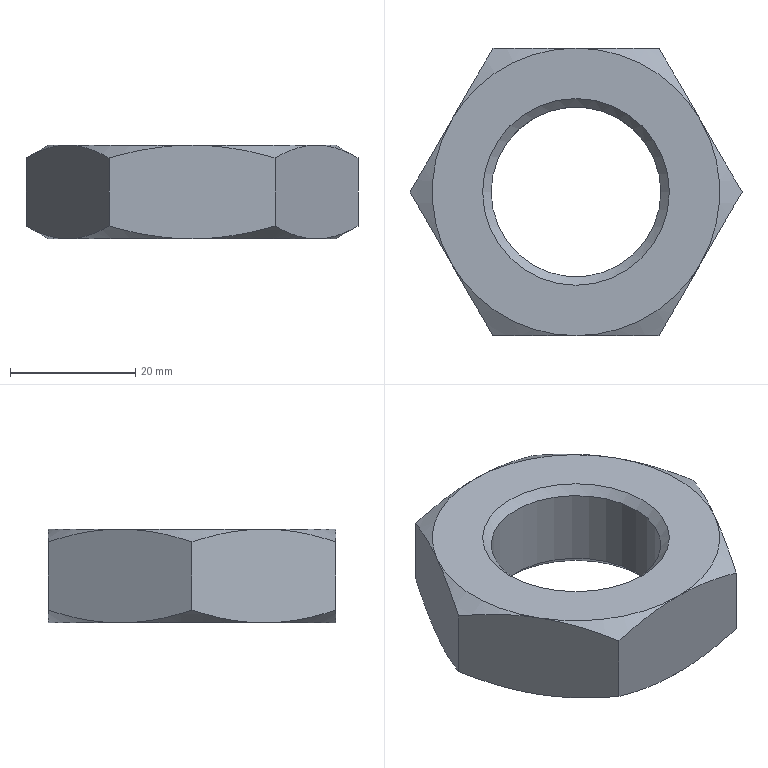Part | NX | features META 3, SKETCH 3, DATUM_CSYS 2, EXTRUDE 2, SWP104 2, CHAMFER 1, LINE 1, SYMBOLIC_THREAD 1, THREADS 1 | 1 solid | 23 faces | box 53.116 x 46 x 15 mm | volume 18421 mm3 | cone 14 | plane 8 | cylinder 1 | commonest cylinder face diameters 27.158 x1
STEP:
#1=CARTESIAN_POINT('',(14.937,0.,15.));
#2=VERTEX_POINT('',#1);
#3=CARTESIAN_POINT('',(0.,0.,15.));
#4=DIRECTION('',(0.,0.,1.));
#5=DIRECTION('',(1.,0.,0.));
#6=AXIS2_PLACEMENT_3D('',#3,#4,#5);
#7=CIRCLE('',#6,14.937);
#8=EDGE_CURVE('',#2,#2,#7,.F.);
#9=ORIENTED_EDGE('',*,*,#8,.T.);
#10=EDGE_LOOP('',(#9));
#11=FACE_BOUND('',#10,.T.);
#12=CARTESIAN_POINT('',(-19.919,11.5,15.));
#13=VERTEX_POINT('',#12);
#14=CARTESIAN_POINT('',(0.,23.,15.));
#15=VERTEX_POINT('',#14);
#16=CARTESIAN_POINT('',(0.,0.,15.));
#17=DIRECTION('',(0.,0.,-1.));
#18=DIRECTION('',(-1.,0.,0.));
#19=AXIS2_PLACEMENT_3D('',#16,#17,#18);
#20=CIRCLE('',#19,23.);
#21=EDGE_CURVE('',#13,#15,#20,.T.);
#22=ORIENTED_EDGE('',*,*,#21,.F.);
#23=CARTESIAN_POINT('',(-19.919,-11.5,15.));
#24=VERTEX_POINT('',#23);
#25=CARTESIAN_POINT('',(0.,0.,15.));
#26=DIRECTION('',(0.,0.,-1.));
#27=DIRECTION('',(-1.,0.,0.));
#28=AXIS2_PLACEMENT_3D('',#25,#26,#27);
#29=CIRCLE('',#28,23.);
#30=EDGE_CURVE('',#24,#13,#29,.T.);
#31=ORIENTED_EDGE('',*,*,#30,.F.);
#32=CARTESIAN_POINT('',(0.,-23.,15.));
#33=VERTEX_POINT('',#32);
#34=CARTESIAN_POINT('',(0.,0.,15.));
#35=DIRECTION('',(0.,0.,-1.));
#36=DIRECTION('',(-1.,0.,0.));
#37=AXIS2_PLACEMENT_3D('',#34,#35,#36);
#38=CIRCLE('',#37,23.);
#39=EDGE_CURVE('',#33,#24,#38,.T.);
#40=ORIENTED_EDGE('',*,*,#39,.F.);
#41=CARTESIAN_POINT('',(19.919,-11.5,15.));
#42=VERTEX_POINT('',#41);
#43=CARTESIAN_POINT('',(0.,0.,15.));
#44=DIRECTION('',(0.,0.,-1.));
#45=DIRECTION('',(-1.,0.,0.));
#46=AXIS2_PLACEMENT_3D('',#43,#44,#45);
#47=CIRCLE('',#46,23.);
#48=EDGE_CURVE('',#42,#33,#47,.T.);
#49=ORIENTED_EDGE('',*,*,#48,.F.);
#50=CARTESIAN_POINT('',(19.919,11.5,15.));
#51=VERTEX_POINT('',#50);
#52=CARTESIAN_POINT('',(0.,0.,15.));
#53=DIRECTION('',(0.,0.,-1.));
#54=DIRECTION('',(-1.,0.,0.));
#55=AXIS2_PLACEMENT_3D('',#52,#53,#54);
#56=CIRCLE('',#55,23.);
#57=EDGE_CURVE('',#51,#42,#56,.T.);
#58=ORIENTED_EDGE('',*,*,#57,.F.);
#59=CARTESIAN_POINT('',(0.,0.,15.));
#60=DIRECTION('',(0.,0.,-1.));
#61=DIRECTION('',(-1.,0.,0.));
#62=AXIS2_PLACEMENT_3D('',#59,#60,#61);
#63=CIRCLE('',#62,23.);
#64=EDGE_CURVE('',#15,#51,#63,.T.);
#65=ORIENTED_EDGE('',*,*,#64,.F.);
#66=EDGE_LOOP('',(#22,#31,#40,#49,#58,#65));
#67=FACE_BOUND('',#66,.T.);
#68=CARTESIAN_POINT('',(0.,46.,15.));
#69=DIRECTION('',(0.,0.,1.));
#70=DIRECTION('',(1.,0.,0.));
#71=AXIS2_PLACEMENT_3D('',#68,#69,#70);
#72=PLANE('',#71);
#73=ADVANCED_FACE('',(#11,#67),#72,.T.);
#74=CARTESIAN_POINT('',(14.937,0.,0.));
#75=VERTEX_POINT('',#74);
#76=CARTESIAN_POINT('',(0.,0.,0.));
#77=DIRECTION('',(0.,0.,1.));
#78=DIRECTION('',(1.,0.,0.));
#79=AXIS2_PLACEMENT_3D('',#76,#77,#78);
#80=CIRCLE('',#79,14.937);
#81=EDGE_CURVE('',#75,#75,#80,.T.);
#82=ORIENTED_EDGE('',*,*,#81,.T.);
#83=EDGE_LOOP('',(#82));
#84=FACE_BOUND('',#83,.T.);
#85=CARTESIAN_POINT('',(-19.919,-11.5,0.));
#86=VERTEX_POINT('',#85);
#87=CARTESIAN_POINT('',(-19.919,11.5,0.));
#88=VERTEX_POINT('',#87);
#89=CARTESIAN_POINT('',(0.,0.,0.));
#90=DIRECTION('',(0.,0.,-1.));
#91=DIRECTION('',(-1.,0.,0.));
#92=AXIS2_PLACEMENT_3D('',#89,#90,#91);
#93=CIRCLE('',#92,23.);
#94=EDGE_CURVE('',#86,#88,#93,.T.);
#95=ORIENTED_EDGE('',*,*,#94,.T.);
#96=CARTESIAN_POINT('',(0.,23.,0.));
#97=VERTEX_POINT('',#96);
#98=CARTESIAN_POINT('',(0.,0.,0.));
#99=DIRECTION('',(0.,0.,-1.));
#100=DIRECTION('',(-1.,0.,0.));
#101=AXIS2_PLACEMENT_3D('',#98,#99,#100);
#102=CIRCLE('',#101,23.);
#103=EDGE_CURVE('',#88,#97,#102,.T.);
#104=ORIENTED_EDGE('',*,*,#103,.T.);
#105=CARTESIAN_POINT('',(19.919,11.5,0.));
#106=VERTEX_POINT('',#105);
#107=CARTESIAN_POINT('',(0.,0.,0.));
#108=DIRECTION('',(0.,0.,-1.));
#109=DIRECTION('',(-1.,0.,0.));
#110=AXIS2_PLACEMENT_3D('',#107,#108,#109);
#111=CIRCLE('',#110,23.);
#112=EDGE_CURVE('',#97,#106,#111,.T.);
#113=ORIENTED_EDGE('',*,*,#112,.T.);
#114=CARTESIAN_POINT('',(19.919,-11.5,0.));
#115=VERTEX_POINT('',#114);
#116=CARTESIAN_POINT('',(0.,0.,0.));
#117=DIRECTION('',(0.,0.,-1.));
#118=DIRECTION('',(-1.,0.,0.));
#119=AXIS2_PLACEMENT_3D('',#116,#117,#118);
#120=CIRCLE('',#119,23.);
#121=EDGE_CURVE('',#106,#115,#120,.T.);
#122=ORIENTED_EDGE('',*,*,#121,.T.);
#123=CARTESIAN_POINT('',(0.,-23.,0.));
#124=VERTEX_POINT('',#123);
#125=CARTESIAN_POINT('',(0.,0.,0.));
#126=DIRECTION('',(0.,0.,-1.));
#127=DIRECTION('',(-1.,0.,0.));
#128=AXIS2_PLACEMENT_3D('',#125,#126,#127);
#129=CIRCLE('',#128,23.);
#130=EDGE_CURVE('',#115,#124,#129,.T.);
#131=ORIENTED_EDGE('',*,*,#130,.T.);
#132=CARTESIAN_POINT('',(0.,0.,0.));
#133=DIRECTION('',(0.,0.,-1.));
#134=DIRECTION('',(-1.,0.,0.));
#135=AXIS2_PLACEMENT_3D('',#132,#133,#134);
#136=CIRCLE('',#135,23.);
#137=EDGE_CURVE('',#124,#86,#136,.T.);
#138=ORIENTED_EDGE('',*,*,#137,.T.);
#139=EDGE_LOOP('',(#95,#104,#113,#122,#131,#138));
#140=FACE_BOUND('',#139,.T.);
#141=CARTESIAN_POINT('',(0.,46.,0.));
#142=DIRECTION('',(0.,0.,1.));
#143=DIRECTION('',(1.,0.,0.));
#144=AXIS2_PLACEMENT_3D('',#141,#142,#143);
#145=PLANE('',#144);
#146=ADVANCED_FACE('',(#84,#140),#145,.F.);
#147=CARTESIAN_POINT('',(26.558,0.,12.946));
#148=VERTEX_POINT('',#147);
#149=CARTESIAN_POINT('',(26.558,0.,2.054));
#150=VERTEX_POINT('',#149);
#151=CARTESIAN_POINT('',(26.558,0.,15.));
#152=DIRECTION('',(0.,0.,-1.));
#153=VECTOR('',#152,1000.);
#154=LINE('',#151,#153);
#155=EDGE_CURVE('',#148,#150,#154,.T.);
#156=ORIENTED_EDGE('',*,*,#155,.T.);
#157=CARTESIAN_POINT('',(26.558,0.,2.054));
#158=CARTESIAN_POINT('',(24.386,3.763,0.8001));
#159=CARTESIAN_POINT('',(22.181,7.581,0.));
#160=CARTESIAN_POINT('',(19.919,11.5,0.));
#161=B_SPLINE_CURVE_WITH_KNOTS('',3,(#157,#158,#159,#160),.UNSPECIFIED.,.F.,.F.,(4,4),(0.000000238,0.01344),.UNSPECIFIED.);
#162=EDGE_CURVE('',#150,#106,#161,.T.);
#163=ORIENTED_EDGE('',*,*,#162,.T.);
#164=CARTESIAN_POINT('',(13.279,23.,2.054));
#165=VERTEX_POINT('',#164);
#166=CARTESIAN_POINT('',(19.919,11.5,0.));
#167=CARTESIAN_POINT('',(17.665,15.404,0.));
#168=CARTESIAN_POINT('',(15.446,19.247,0.8032));
#169=CARTESIAN_POINT('',(13.279,23.,2.054));
#170=B_SPLINE_CURVE_WITH_KNOTS('',3,(#166,#167,#168,#169),.UNSPECIFIED.,.F.,.F.,(4,4),(0.01344,0.02682),.UNSPECIFIED.);
#171=EDGE_CURVE('',#106,#165,#170,.T.);
#172=ORIENTED_EDGE('',*,*,#171,.T.);
#173=CARTESIAN_POINT('',(13.279,23.,12.946));
#174=VERTEX_POINT('',#173);
#175=CARTESIAN_POINT('',(13.279,23.,15.));
#176=DIRECTION('',(0.,0.,-1.));
#177=VECTOR('',#176,1000.);
#178=LINE('',#175,#177);
#179=EDGE_CURVE('',#174,#165,#178,.T.);
#180=ORIENTED_EDGE('',*,*,#179,.F.);
#181=CARTESIAN_POINT('',(13.279,23.,12.946));
#182=CARTESIAN_POINT('',(15.451,19.237,14.2));
#183=CARTESIAN_POINT('',(17.656,15.419,15.));
#184=CARTESIAN_POINT('',(19.919,11.5,15.));
#185=B_SPLINE_CURVE_WITH_KNOTS('',3,(#181,#182,#183,#184),.UNSPECIFIED.,.F.,.F.,(4,4),(0.000000238,0.01344),.UNSPECIFIED.);
#186=EDGE_CURVE('',#174,#51,#185,.T.);
#187=ORIENTED_EDGE('',*,*,#186,.T.);
#188=CARTESIAN_POINT('',(19.919,11.5,15.));
#189=CARTESIAN_POINT('',(22.172,7.596,15.));
#190=CARTESIAN_POINT('',(24.391,3.753,14.197));
#191=CARTESIAN_POINT('',(26.558,0.,12.946));
#192=B_SPLINE_CURVE_WITH_KNOTS('',3,(#188,#189,#190,#191),.UNSPECIFIED.,.F.,.F.,(4,4),(0.01344,0.02682),.UNSPECIFIED.);
#193=EDGE_CURVE('',#51,#148,#192,.T.);
#194=ORIENTED_EDGE('',*,*,#193,.T.);
#195=EDGE_LOOP('',(#156,#163,#172,#180,#187,#194));
#196=FACE_BOUND('',#195,.T.);
#197=CARTESIAN_POINT('',(13.279,23.,15.));
#198=DIRECTION('',(0.866,0.5,0.));
#199=DIRECTION('',(-0.5,0.866,0.));
#200=AXIS2_PLACEMENT_3D('',#197,#198,#199);
#201=PLANE('',#200);
#202=ADVANCED_FACE('',(#196),#201,.T.);
#203=CARTESIAN_POINT('',(13.279,-23.,12.946));
#204=VERTEX_POINT('',#203);
#205=CARTESIAN_POINT('',(13.279,-23.,2.054));
#206=VERTEX_POINT('',#205);
#207=CARTESIAN_POINT('',(13.279,-23.,15.));
#208=DIRECTION('',(0.,0.,-1.));
#209=VECTOR('',#208,1000.);
#210=LINE('',#207,#209);
#211=EDGE_CURVE('',#204,#206,#210,.T.);
#212=ORIENTED_EDGE('',*,*,#211,.T.);
#213=CARTESIAN_POINT('',(13.279,-23.,2.054));
#214=CARTESIAN_POINT('',(15.451,-19.237,0.8001));
#215=CARTESIAN_POINT('',(17.656,-15.419,0.));
#216=CARTESIAN_POINT('',(19.919,-11.5,0.));
#217=B_SPLINE_CURVE_WITH_KNOTS('',3,(#213,#214,#215,#216),.UNSPECIFIED.,.F.,.F.,(4,4),(0.000000238,0.01344),.UNSPECIFIED.);
#218=EDGE_CURVE('',#206,#115,#217,.T.);
#219=ORIENTED_EDGE('',*,*,#218,.T.);
#220=CARTESIAN_POINT('',(19.919,-11.5,0.));
#221=CARTESIAN_POINT('',(22.172,-7.596,0.));
#222=CARTESIAN_POINT('',(24.391,-3.753,0.8032));
#223=CARTESIAN_POINT('',(26.558,0.,2.054));
#224=B_SPLINE_CURVE_WITH_KNOTS('',3,(#220,#221,#222,#223),.UNSPECIFIED.,.F.,.F.,(4,4),(0.01344,0.02682),.UNSPECIFIED.);
#225=EDGE_CURVE('',#115,#150,#224,.T.);
#226=ORIENTED_EDGE('',*,*,#225,.T.);
#227=ORIENTED_EDGE('',*,*,#155,.F.);
#228=CARTESIAN_POINT('',(26.558,0.,12.946));
#229=CARTESIAN_POINT('',(24.386,-3.763,14.2));
#230=CARTESIAN_POINT('',(22.181,-7.581,15.));
#231=CARTESIAN_POINT('',(19.919,-11.5,15.));
#232=B_SPLINE_CURVE_WITH_KNOTS('',3,(#228,#229,#230,#231),.UNSPECIFIED.,.F.,.F.,(4,4),(0.000000238,0.01344),.UNSPECIFIED.);
#233=EDGE_CURVE('',#148,#42,#232,.T.);
#234=ORIENTED_EDGE('',*,*,#233,.T.);
#235=CARTESIAN_POINT('',(19.919,-11.5,15.));
#236=CARTESIAN_POINT('',(17.665,-15.404,15.));
#237=CARTESIAN_POINT('',(15.446,-19.247,14.197));
#238=CARTESIAN_POINT('',(13.279,-23.,12.946));
#239=B_SPLINE_CURVE_WITH_KNOTS('',3,(#235,#236,#237,#238),.UNSPECIFIED.,.F.,.F.,(4,4),(0.01344,0.02682),.UNSPECIFIED.);
#240=EDGE_CURVE('',#42,#204,#239,.T.);
#241=ORIENTED_EDGE('',*,*,#240,.T.);
#242=EDGE_LOOP('',(#212,#219,#226,#227,#234,#241));
#243=FACE_BOUND('',#242,.T.);
#244=CARTESIAN_POINT('',(26.558,0.,15.));
#245=DIRECTION('',(0.866,-0.5,0.));
#246=DIRECTION('',(0.5,0.866,0.));
#247=AXIS2_PLACEMENT_3D('',#244,#245,#246);
#248=PLANE('',#247);
#249=ADVANCED_FACE('',(#243),#248,.T.);
#250=CARTESIAN_POINT('',(-13.279,-23.,12.946));
#251=VERTEX_POINT('',#250);
#252=CARTESIAN_POINT('',(-13.279,-23.,2.054));
#253=VERTEX_POINT('',#252);
#254=CARTESIAN_POINT('',(-13.279,-23.,15.));
#255=DIRECTION('',(0.,0.,-1.));
#256=VECTOR('',#255,1000.);
#257=LINE('',#254,#256);
#258=EDGE_CURVE('',#251,#253,#257,.T.);
#259=ORIENTED_EDGE('',*,*,#258,.T.);
#260=CARTESIAN_POINT('',(-13.279,-23.,2.054));
#261=CARTESIAN_POINT('',(-8.96,-23.,0.8074));
#262=CARTESIAN_POINT('',(-4.488,-23.,0.));
#263=CARTESIAN_POINT('',(0.,-23.,0.));
#264=B_SPLINE_CURVE_WITH_KNOTS('',3,(#260,#261,#262,#263),.UNSPECIFIED.,.F.,.F.,(4,4),(0.02369,0.03713),.UNSPECIFIED.);
#265=EDGE_CURVE('',#253,#124,#264,.T.);
#266=ORIENTED_EDGE('',*,*,#265,.T.);
#267=CARTESIAN_POINT('',(0.,-23.,0.));
#268=CARTESIAN_POINT('',(2.245,-23.,0.));
#269=CARTESIAN_POINT('',(6.789,-23.,0.3992));
#270=CARTESIAN_POINT('',(11.132,-23.,1.434));
#271=CARTESIAN_POINT('',(13.279,-23.,2.054));
#272=B_SPLINE_CURVE_WITH_KNOTS('',3,(#267,#268,#269,#270,#271),.UNSPECIFIED.,.F.,.F.,(4,1,4),(0.03713,0.04385,0.05057),.UNSPECIFIED.);
#273=EDGE_CURVE('',#124,#206,#272,.T.);
#274=ORIENTED_EDGE('',*,*,#273,.T.);
#275=ORIENTED_EDGE('',*,*,#211,.F.);
#276=CARTESIAN_POINT('',(0.,-23.,15.));
#277=CARTESIAN_POINT('',(2.245,-23.,15.));
#278=CARTESIAN_POINT('',(6.789,-23.,14.601));
#279=CARTESIAN_POINT('',(11.132,-23.,13.566));
#280=CARTESIAN_POINT('',(13.279,-23.,12.946));
#281=B_SPLINE_CURVE_WITH_KNOTS('',3,(#276,#277,#278,#279,#280),.UNSPECIFIED.,.F.,.F.,(4,1,4),(0.03713,0.04385,0.05057),.UNSPECIFIED.);
#282=EDGE_CURVE('',#204,#33,#281,.F.);
#283=ORIENTED_EDGE('',*,*,#282,.T.);
#284=CARTESIAN_POINT('',(-13.279,-23.,12.946));
#285=CARTESIAN_POINT('',(-8.96,-23.,14.193));
#286=CARTESIAN_POINT('',(-4.488,-23.,15.));
#287=CARTESIAN_POINT('',(0.,-23.,15.));
#288=B_SPLINE_CURVE_WITH_KNOTS('',3,(#284,#285,#286,#287),.UNSPECIFIED.,.F.,.F.,(4,4),(0.02369,0.03713),.UNSPECIFIED.);
#289=EDGE_CURVE('',#33,#251,#288,.F.);
#290=ORIENTED_EDGE('',*,*,#289,.T.);
#291=EDGE_LOOP('',(#259,#266,#274,#275,#283,#290));
#292=FACE_BOUND('',#291,.T.);
#293=CARTESIAN_POINT('',(13.279,-23.,15.));
#294=DIRECTION('',(0.,-1.,0.));
#295=DIRECTION('',(1.,0.,0.));
#296=AXIS2_PLACEMENT_3D('',#293,#294,#295);
#297=PLANE('',#296);
#298=ADVANCED_FACE('',(#292),#297,.T.);
#299=CARTESIAN_POINT('',(-26.558,0.,12.946));
#300=VERTEX_POINT('',#299);
#301=CARTESIAN_POINT('',(-26.558,0.,2.054));
#302=VERTEX_POINT('',#301);
#303=CARTESIAN_POINT('',(-26.558,0.,15.));
#304=DIRECTION('',(0.,0.,-1.));
#305=VECTOR('',#304,1000.);
#306=LINE('',#303,#305);
#307=EDGE_CURVE('',#300,#302,#306,.T.);
#308=ORIENTED_EDGE('',*,*,#307,.T.);
#309=CARTESIAN_POINT('',(-26.558,0.,2.054));
#310=CARTESIAN_POINT('',(-24.386,-3.763,0.8001));
#311=CARTESIAN_POINT('',(-22.181,-7.581,0.));
#312=CARTESIAN_POINT('',(-19.919,-11.5,0.));
#313=B_SPLINE_CURVE_WITH_KNOTS('',3,(#309,#310,#311,#312),.UNSPECIFIED.,.F.,.F.,(4,4),(0.000000238,0.01344),.UNSPECIFIED.);
#314=EDGE_CURVE('',#302,#86,#313,.T.);
#315=ORIENTED_EDGE('',*,*,#314,.T.);
#316=CARTESIAN_POINT('',(-19.919,-11.5,0.));
#317=CARTESIAN_POINT('',(-17.665,-15.404,0.));
#318=CARTESIAN_POINT('',(-15.446,-19.247,0.8032));
#319=CARTESIAN_POINT('',(-13.279,-23.,2.054));
#320=B_SPLINE_CURVE_WITH_KNOTS('',3,(#316,#317,#318,#319),.UNSPECIFIED.,.F.,.F.,(4,4),(0.01344,0.02682),.UNSPECIFIED.);
#321=EDGE_CURVE('',#86,#253,#320,.T.);
#322=ORIENTED_EDGE('',*,*,#321,.T.);
#323=ORIENTED_EDGE('',*,*,#258,.F.);
#324=CARTESIAN_POINT('',(-13.279,-23.,12.946));
#325=CARTESIAN_POINT('',(-15.451,-19.237,14.2));
#326=CARTESIAN_POINT('',(-17.656,-15.419,15.));
#327=CARTESIAN_POINT('',(-19.919,-11.5,15.));
#328=B_SPLINE_CURVE_WITH_KNOTS('',3,(#324,#325,#326,#327),.UNSPECIFIED.,.F.,.F.,(4,4),(0.000000238,0.01344),.UNSPECIFIED.);
#329=EDGE_CURVE('',#251,#24,#328,.T.);
#330=ORIENTED_EDGE('',*,*,#329,.T.);
#331=CARTESIAN_POINT('',(-19.919,-11.5,15.));
#332=CARTESIAN_POINT('',(-22.172,-7.596,15.));
#333=CARTESIAN_POINT('',(-24.391,-3.753,14.197));
#334=CARTESIAN_POINT('',(-26.558,0.,12.946));
#335=B_SPLINE_CURVE_WITH_KNOTS('',3,(#331,#332,#333,#334),.UNSPECIFIED.,.F.,.F.,(4,4),(0.01344,0.02682),.UNSPECIFIED.);
#336=EDGE_CURVE('',#24,#300,#335,.T.);
#337=ORIENTED_EDGE('',*,*,#336,.T.);
#338=EDGE_LOOP('',(#308,#315,#322,#323,#330,#337));
#339=FACE_BOUND('',#338,.T.);
#340=CARTESIAN_POINT('',(-13.279,-23.,15.));
#341=DIRECTION('',(-0.866,-0.5,0.));
#342=DIRECTION('',(0.5,-0.866,0.));
#343=AXIS2_PLACEMENT_3D('',#340,#341,#342);
#344=PLANE('',#343);
#345=ADVANCED_FACE('',(#339),#344,.T.);
#346=CARTESIAN_POINT('',(-13.279,23.,12.946));
#347=VERTEX_POINT('',#346);
#348=CARTESIAN_POINT('',(-13.279,23.,2.054));
#349=VERTEX_POINT('',#348);
#350=CARTESIAN_POINT('',(-13.279,23.,15.));
#351=DIRECTION('',(0.,0.,-1.));
#352=VECTOR('',#351,1000.);
#353=LINE('',#350,#352);
#354=EDGE_CURVE('',#347,#349,#353,.T.);
#355=ORIENTED_EDGE('',*,*,#354,.T.);
#356=CARTESIAN_POINT('',(-13.279,23.,2.054));
#357=CARTESIAN_POINT('',(-15.451,19.237,0.8001));
#358=CARTESIAN_POINT('',(-17.656,15.419,0.));
#359=CARTESIAN_POINT('',(-19.919,11.5,0.));
#360=B_SPLINE_CURVE_WITH_KNOTS('',3,(#356,#357,#358,#359),.UNSPECIFIED.,.F.,.F.,(4,4),(0.000000238,0.01344),.UNSPECIFIED.);
#361=EDGE_CURVE('',#349,#88,#360,.T.);
#362=ORIENTED_EDGE('',*,*,#361,.T.);
#363=CARTESIAN_POINT('',(-19.919,11.5,0.));
#364=CARTESIAN_POINT('',(-22.172,7.596,0.));
#365=CARTESIAN_POINT('',(-24.391,3.753,0.8032));
#366=CARTESIAN_POINT('',(-26.558,0.,2.054));
#367=B_SPLINE_CURVE_WITH_KNOTS('',3,(#363,#364,#365,#366),.UNSPECIFIED.,.F.,.F.,(4,4),(0.01344,0.02682),.UNSPECIFIED.);
#368=EDGE_CURVE('',#88,#302,#367,.T.);
#369=ORIENTED_EDGE('',*,*,#368,.T.);
#370=ORIENTED_EDGE('',*,*,#307,.F.);
#371=CARTESIAN_POINT('',(-26.558,0.,12.946));
#372=CARTESIAN_POINT('',(-24.386,3.763,14.2));
#373=CARTESIAN_POINT('',(-22.181,7.581,15.));
#374=CARTESIAN_POINT('',(-19.919,11.5,15.));
#375=B_SPLINE_CURVE_WITH_KNOTS('',3,(#371,#372,#373,#374),.UNSPECIFIED.,.F.,.F.,(4,4),(0.000000238,0.01344),.UNSPECIFIED.);
#376=EDGE_CURVE('',#300,#13,#375,.T.);
#377=ORIENTED_EDGE('',*,*,#376,.T.);
#378=CARTESIAN_POINT('',(-19.919,11.5,15.));
#379=CARTESIAN_POINT('',(-17.665,15.404,15.));
#380=CARTESIAN_POINT('',(-15.446,19.247,14.197));
#381=CARTESIAN_POINT('',(-13.279,23.,12.946));
#382=B_SPLINE_CURVE_WITH_KNOTS('',3,(#378,#379,#380,#381),.UNSPECIFIED.,.F.,.F.,(4,4),(0.01344,0.02682),.UNSPECIFIED.);
#383=EDGE_CURVE('',#13,#347,#382,.T.);
#384=ORIENTED_EDGE('',*,*,#383,.T.);
#385=EDGE_LOOP('',(#355,#362,#369,#370,#377,#384));
#386=FACE_BOUND('',#385,.T.);
#387=CARTESIAN_POINT('',(-26.558,0.,15.));
#388=DIRECTION('',(-0.866,0.5,0.));
#389=DIRECTION('',(-0.5,-0.866,0.));
#390=AXIS2_PLACEMENT_3D('',#387,#388,#389);
#391=PLANE('',#390);
#392=ADVANCED_FACE('',(#386),#391,.T.);
#393=ORIENTED_EDGE('',*,*,#179,.T.);
#394=CARTESIAN_POINT('',(0.,23.,0.));
#395=CARTESIAN_POINT('',(2.245,23.,0.));
#396=CARTESIAN_POINT('',(6.789,23.,0.3992));
#397=CARTESIAN_POINT('',(11.132,23.,1.434));
#398=CARTESIAN_POINT('',(13.279,23.,2.054));
#399=B_SPLINE_CURVE_WITH_KNOTS('',3,(#394,#395,#396,#397,#398),.UNSPECIFIED.,.F.,.F.,(4,1,4),(0.03713,0.04385,0.05057),.UNSPECIFIED.);
#400=EDGE_CURVE('',#165,#97,#399,.F.);
#401=ORIENTED_EDGE('',*,*,#400,.T.);
#402=CARTESIAN_POINT('',(-13.279,23.,2.054));
#403=CARTESIAN_POINT('',(-8.96,23.,0.8074));
#404=CARTESIAN_POINT('',(-4.488,23.,0.));
#405=CARTESIAN_POINT('',(0.,23.,0.));
#406=B_SPLINE_CURVE_WITH_KNOTS('',3,(#402,#403,#404,#405),.UNSPECIFIED.,.F.,.F.,(4,4),(0.02369,0.03713),.UNSPECIFIED.);
#407=EDGE_CURVE('',#97,#349,#406,.F.);
#408=ORIENTED_EDGE('',*,*,#407,.T.);
#409=ORIENTED_EDGE('',*,*,#354,.F.);
#410=CARTESIAN_POINT('',(-13.279,23.,12.946));
#411=CARTESIAN_POINT('',(-8.96,23.,14.193));
#412=CARTESIAN_POINT('',(-4.488,23.,15.));
#413=CARTESIAN_POINT('',(0.,23.,15.));
#414=B_SPLINE_CURVE_WITH_KNOTS('',3,(#410,#411,#412,#413),.UNSPECIFIED.,.F.,.F.,(4,4),(0.02369,0.03713),.UNSPECIFIED.);
#415=EDGE_CURVE('',#347,#15,#414,.T.);
#416=ORIENTED_EDGE('',*,*,#415,.T.);
#417=CARTESIAN_POINT('',(0.,23.,15.));
#418=CARTESIAN_POINT('',(2.245,23.,15.));
#419=CARTESIAN_POINT('',(6.789,23.,14.601));
#420=CARTESIAN_POINT('',(11.132,23.,13.566));
#421=CARTESIAN_POINT('',(13.279,23.,12.946));
#422=B_SPLINE_CURVE_WITH_KNOTS('',3,(#417,#418,#419,#420,#421),.UNSPECIFIED.,.F.,.F.,(4,1,4),(0.03713,0.04385,0.05057),.UNSPECIFIED.);
#423=EDGE_CURVE('',#15,#174,#422,.T.);
#424=ORIENTED_EDGE('',*,*,#423,.T.);
#425=EDGE_LOOP('',(#393,#401,#408,#409,#416,#424));
#426=FACE_BOUND('',#425,.T.);
#427=CARTESIAN_POINT('',(-13.279,23.,15.));
#428=DIRECTION('',(0.,1.,0.));
#429=DIRECTION('',(-1.,0.,0.));
#430=AXIS2_PLACEMENT_3D('',#427,#428,#429);
#431=PLANE('',#430);
#432=ADVANCED_FACE('',(#426),#431,.T.);
#433=ORIENTED_EDGE('',*,*,#423,.F.);
#434=ORIENTED_EDGE('',*,*,#64,.T.);
#435=ORIENTED_EDGE('',*,*,#186,.F.);
#436=EDGE_LOOP('',(#433,#434,#435));
#437=FACE_BOUND('',#436,.T.);
#438=CARTESIAN_POINT('',(0.,0.,12.946));
#439=DIRECTION('',(0.,0.,-1.));
#440=DIRECTION('',(-1.,0.,0.));
#441=AXIS2_PLACEMENT_3D('',#438,#439,#440);
#442=CONICAL_SURFACE('',#441,26.558,1.047);
#443=ADVANCED_FACE('',(#437),#442,.T.);
#444=ORIENTED_EDGE('',*,*,#21,.T.);
#445=ORIENTED_EDGE('',*,*,#415,.F.);
#446=ORIENTED_EDGE('',*,*,#383,.F.);
#447=EDGE_LOOP('',(#444,#445,#446));
#448=FACE_BOUND('',#447,.T.);
#449=CARTESIAN_POINT('',(0.,0.,12.946));
#450=DIRECTION('',(0.,0.,-1.));
#451=DIRECTION('',(-1.,0.,0.));
#452=AXIS2_PLACEMENT_3D('',#449,#450,#451);
#453=CONICAL_SURFACE('',#452,26.558,1.047);
#454=ADVANCED_FACE('',(#448),#453,.T.);
#455=ORIENTED_EDGE('',*,*,#30,.T.);
#456=ORIENTED_EDGE('',*,*,#376,.F.);
#457=ORIENTED_EDGE('',*,*,#336,.F.);
#458=EDGE_LOOP('',(#455,#456,#457));
#459=FACE_BOUND('',#458,.T.);
#460=CARTESIAN_POINT('',(0.,0.,12.946));
#461=DIRECTION('',(0.,0.,-1.));
#462=DIRECTION('',(-1.,0.,0.));
#463=AXIS2_PLACEMENT_3D('',#460,#461,#462);
#464=CONICAL_SURFACE('',#463,26.558,1.047);
#465=ADVANCED_FACE('',(#459),#464,.T.);
#466=ORIENTED_EDGE('',*,*,#39,.T.);
#467=ORIENTED_EDGE('',*,*,#329,.F.);
#468=ORIENTED_EDGE('',*,*,#289,.F.);
#469=EDGE_LOOP('',(#466,#467,#468));
#470=FACE_BOUND('',#469,.T.);
#471=CARTESIAN_POINT('',(0.,0.,12.946));
#472=DIRECTION('',(0.,0.,-1.));
#473=DIRECTION('',(-1.,0.,0.));
#474=AXIS2_PLACEMENT_3D('',#471,#472,#473);
#475=CONICAL_SURFACE('',#474,26.558,1.047);
#476=ADVANCED_FACE('',(#470),#475,.T.);
#477=ORIENTED_EDGE('',*,*,#48,.T.);
#478=ORIENTED_EDGE('',*,*,#282,.F.);
#479=ORIENTED_EDGE('',*,*,#240,.F.);
#480=EDGE_LOOP('',(#477,#478,#479));
#481=FACE_BOUND('',#480,.T.);
#482=CARTESIAN_POINT('',(0.,0.,12.946));
#483=DIRECTION('',(0.,0.,-1.));
#484=DIRECTION('',(-1.,0.,0.));
#485=AXIS2_PLACEMENT_3D('',#482,#483,#484);
#486=CONICAL_SURFACE('',#485,26.558,1.047);
#487=ADVANCED_FACE('',(#481),#486,.T.);
#488=ORIENTED_EDGE('',*,*,#57,.T.);
#489=ORIENTED_EDGE('',*,*,#233,.F.);
#490=ORIENTED_EDGE('',*,*,#193,.F.);
#491=EDGE_LOOP('',(#488,#489,#490));
#492=FACE_BOUND('',#491,.T.);
#493=CARTESIAN_POINT('',(0.,0.,12.946));
#494=DIRECTION('',(0.,0.,-1.));
#495=DIRECTION('',(-1.,0.,0.));
#496=AXIS2_PLACEMENT_3D('',#493,#494,#495);
#497=CONICAL_SURFACE('',#496,26.558,1.047);
#498=ADVANCED_FACE('',(#492),#497,.T.);
#499=ORIENTED_EDGE('',*,*,#407,.F.);
#500=ORIENTED_EDGE('',*,*,#103,.F.);
#501=ORIENTED_EDGE('',*,*,#361,.F.);
#502=EDGE_LOOP('',(#499,#500,#501));
#503=FACE_BOUND('',#502,.T.);
#504=CARTESIAN_POINT('',(0.,0.,0.));
#505=DIRECTION('',(0.,0.,1.));
#506=DIRECTION('',(1.,0.,0.));
#507=AXIS2_PLACEMENT_3D('',#504,#505,#506);
#508=CONICAL_SURFACE('',#507,23.,1.047);
#509=ADVANCED_FACE('',(#503),#508,.T.);
#510=ORIENTED_EDGE('',*,*,#112,.F.);
#511=ORIENTED_EDGE('',*,*,#400,.F.);
#512=ORIENTED_EDGE('',*,*,#171,.F.);
#513=EDGE_LOOP('',(#510,#511,#512));
#514=FACE_BOUND('',#513,.T.);
#515=CARTESIAN_POINT('',(0.,0.,0.));
#516=DIRECTION('',(0.,0.,1.));
#517=DIRECTION('',(1.,0.,0.));
#518=AXIS2_PLACEMENT_3D('',#515,#516,#517);
#519=CONICAL_SURFACE('',#518,23.,1.047);
#520=ADVANCED_FACE('',(#514),#519,.T.);
#521=ORIENTED_EDGE('',*,*,#368,.F.);
#522=ORIENTED_EDGE('',*,*,#94,.F.);
#523=ORIENTED_EDGE('',*,*,#314,.F.);
#524=EDGE_LOOP('',(#521,#522,#523));
#525=FACE_BOUND('',#524,.T.);
#526=CARTESIAN_POINT('',(0.,0.,0.));
#527=DIRECTION('',(0.,0.,1.));
#528=DIRECTION('',(1.,0.,0.));
#529=AXIS2_PLACEMENT_3D('',#526,#527,#528);
#530=CONICAL_SURFACE('',#529,23.,1.047);
#531=ADVANCED_FACE('',(#525),#530,.T.);
#532=ORIENTED_EDGE('',*,*,#321,.F.);
#533=ORIENTED_EDGE('',*,*,#137,.F.);
#534=ORIENTED_EDGE('',*,*,#265,.F.);
#535=EDGE_LOOP('',(#532,#533,#534));
#536=FACE_BOUND('',#535,.T.);
#537=CARTESIAN_POINT('',(0.,0.,0.));
#538=DIRECTION('',(0.,0.,1.));
#539=DIRECTION('',(1.,0.,0.));
#540=AXIS2_PLACEMENT_3D('',#537,#538,#539);
#541=CONICAL_SURFACE('',#540,23.,1.047);
#542=ADVANCED_FACE('',(#536),#541,.T.);
#543=ORIENTED_EDGE('',*,*,#130,.F.);
#544=ORIENTED_EDGE('',*,*,#218,.F.);
#545=ORIENTED_EDGE('',*,*,#273,.F.);
#546=EDGE_LOOP('',(#543,#544,#545));
#547=FACE_BOUND('',#546,.T.);
#548=CARTESIAN_POINT('',(0.,0.,0.));
#549=DIRECTION('',(0.,0.,1.));
#550=DIRECTION('',(1.,0.,0.));
#551=AXIS2_PLACEMENT_3D('',#548,#549,#550);
#552=CONICAL_SURFACE('',#551,23.,1.047);
#553=ADVANCED_FACE('',(#547),#552,.T.);
#554=ORIENTED_EDGE('',*,*,#121,.F.);
#555=ORIENTED_EDGE('',*,*,#162,.F.);
#556=ORIENTED_EDGE('',*,*,#225,.F.);
#557=EDGE_LOOP('',(#554,#555,#556));
#558=FACE_BOUND('',#557,.T.);
#559=CARTESIAN_POINT('',(0.,0.,0.));
#560=DIRECTION('',(0.,0.,1.));
#561=DIRECTION('',(1.,0.,0.));
#562=AXIS2_PLACEMENT_3D('',#559,#560,#561);
#563=CONICAL_SURFACE('',#562,23.,1.047);
#564=ADVANCED_FACE('',(#558),#563,.T.);
#565=CARTESIAN_POINT('',(13.579,0.,1.358));
#566=VERTEX_POINT('',#565);
#567=CARTESIAN_POINT('',(0.,0.,1.358));
#568=DIRECTION('',(0.,0.,1.));
#569=DIRECTION('',(1.,0.,0.));
#570=AXIS2_PLACEMENT_3D('',#567,#568,#569);
#571=CIRCLE('',#570,13.579);
#572=EDGE_CURVE('',#566,#566,#571,.F.);
#573=ORIENTED_EDGE('',*,*,#572,.T.);
#574=EDGE_LOOP('',(#573));
#575=FACE_BOUND('',#574,.T.);
#576=CARTESIAN_POINT('',(13.579,0.,13.642));
#577=VERTEX_POINT('',#576);
#578=CARTESIAN_POINT('',(0.,0.,13.642));
#579=DIRECTION('',(0.,0.,1.));
#580=DIRECTION('',(1.,0.,0.));
#581=AXIS2_PLACEMENT_3D('',#578,#579,#580);
#582=CIRCLE('',#581,13.579);
#583=EDGE_CURVE('',#577,#577,#582,.T.);
#584=ORIENTED_EDGE('',*,*,#583,.T.);
#585=EDGE_LOOP('',(#584));
#586=FACE_BOUND('',#585,.T.);
#587=CARTESIAN_POINT('',(0.,0.,15.));
#588=DIRECTION('',(0.,0.,-1.));
#589=DIRECTION('',(-1.,0.,0.));
#590=AXIS2_PLACEMENT_3D('',#587,#588,#589);
#591=CYLINDRICAL_SURFACE('',#590,13.579);
#592=ADVANCED_FACE('',(#575,#586),#591,.F.);
#593=ORIENTED_EDGE('',*,*,#81,.F.);
#594=EDGE_LOOP('',(#593));
#595=FACE_BOUND('',#594,.T.);
#596=ORIENTED_EDGE('',*,*,#572,.F.);
#597=EDGE_LOOP('',(#596));
#598=FACE_BOUND('',#597,.T.);
#599=CARTESIAN_POINT('',(0.,0.,1.358));
#600=DIRECTION('',(0.,0.,-1.));
#601=DIRECTION('',(-1.,0.,0.));
#602=AXIS2_PLACEMENT_3D('',#599,#600,#601);
#603=CONICAL_SURFACE('',#602,13.579,0.7854);
#604=ADVANCED_FACE('',(#595,#598),#603,.F.);
#605=ORIENTED_EDGE('',*,*,#583,.F.);
#606=EDGE_LOOP('',(#605));
#607=FACE_BOUND('',#606,.T.);
#608=ORIENTED_EDGE('',*,*,#8,.F.);
#609=EDGE_LOOP('',(#608));
#610=FACE_BOUND('',#609,.T.);
#611=CARTESIAN_POINT('',(0.,0.,15.));
#612=DIRECTION('',(0.,0.,1.));
#613=DIRECTION('',(1.,0.,0.));
#614=AXIS2_PLACEMENT_3D('',#611,#612,#613);
#615=CONICAL_SURFACE('',#614,14.937,0.7854);
#616=ADVANCED_FACE('',(#607,#610),#615,.F.);
#617=CLOSED_SHELL('',(#73,#146,#202,#249,#298,#345,#392,#432,#443,#454,#465,#476,#487,#498,#509,#520,#531,#542,#553,#564,#592,#604,#616));
#618=MANIFOLD_SOLID_BREP('',#617);
#619=(LENGTH_UNIT()NAMED_UNIT(*)SI_UNIT(.MILLI.,.METRE.));
#620=UNCERTAINTY_MEASURE_WITH_UNIT(LENGTH_MEASURE(0.0508),#619,'','');
#621=(NAMED_UNIT(*)PLANE_ANGLE_UNIT()SI_UNIT($,.RADIAN.));
#622=(NAMED_UNIT(*)SI_UNIT($,.STERADIAN.)SOLID_ANGLE_UNIT());
#623=(GEOMETRIC_REPRESENTATION_CONTEXT(3)GLOBAL_UNCERTAINTY_ASSIGNED_CONTEXT((#620))GLOBAL_UNIT_ASSIGNED_CONTEXT((#619,#621,#622))REPRESENTATION_CONTEXT('',''));
#624=ADVANCED_BREP_SHAPE_REPRESENTATION('',(#618),#623);